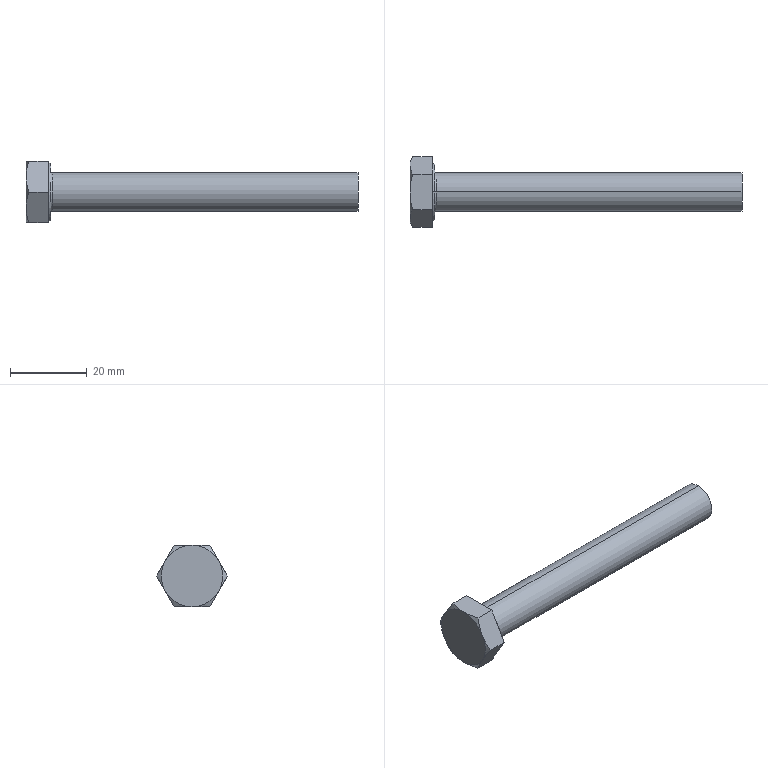Part | SolidWorks | features RevCut 3, Extrusion 1, Fillet 1, LPattern 1, Revolution 1 | 1 solid | 22 faces | box 86.4 x 18.475 x 16 mm | volume 7671 mm3 | plane 10 | cone 8 | torus 2 | cylinder 2 | commonest cylinder face diameters 10 x2
STEP:
#1=CARTESIAN_POINT('',(6.8,0.,5.));
#2=VERTEX_POINT('',#1);
#3=CARTESIAN_POINT('',(6.8,0.,-5.));
#4=VERTEX_POINT('',#3);
#5=CARTESIAN_POINT('',(6.8,0.,0.));
#6=DIRECTION('',(1.,0.,0.));
#7=DIRECTION('',(0.,0.,-1.));
#8=AXIS2_PLACEMENT_3D('',#5,#6,#7);
#9=CIRCLE('',#8,5.);
#10=EDGE_CURVE('',#2,#4,#9,.T.);
#11=ORIENTED_EDGE('',*,*,#10,.F.);
#12=CARTESIAN_POINT('',(6.4,0.,5.4));
#13=VERTEX_POINT('',#12);
#14=CARTESIAN_POINT('',(6.8,0.,5.4));
#15=DIRECTION('',(0.,1.,0.));
#16=DIRECTION('',(0.,0.,1.));
#17=AXIS2_PLACEMENT_3D('',#14,#15,#16);
#18=CIRCLE('',#17,0.4);
#19=EDGE_CURVE('',#2,#13,#18,.T.);
#20=ORIENTED_EDGE('',*,*,#19,.T.);
#21=CARTESIAN_POINT('',(6.4,0.,-5.4));
#22=VERTEX_POINT('',#21);
#23=CARTESIAN_POINT('',(6.4,0.,0.));
#24=DIRECTION('',(-1.,0.,0.));
#25=DIRECTION('',(0.,0.,-1.));
#26=AXIS2_PLACEMENT_3D('',#23,#24,#25);
#27=CIRCLE('',#26,5.4);
#28=EDGE_CURVE('',#22,#13,#27,.T.);
#29=ORIENTED_EDGE('',*,*,#28,.F.);
#30=CARTESIAN_POINT('',(6.8,0.,-5.4));
#31=DIRECTION('',(0.,-1.,0.));
#32=DIRECTION('',(0.,0.,-1.));
#33=AXIS2_PLACEMENT_3D('',#30,#31,#32);
#34=CIRCLE('',#33,0.4);
#35=EDGE_CURVE('',#4,#22,#34,.T.);
#36=ORIENTED_EDGE('',*,*,#35,.F.);
#37=EDGE_LOOP('',(#11,#20,#29,#36));
#38=FACE_OUTER_BOUND('',#37,.T.);
#39=CARTESIAN_POINT('',(6.8,0.,0.));
#40=DIRECTION('',(1.,0.,0.));
#41=DIRECTION('',(0.,0.,-1.));
#42=AXIS2_PLACEMENT_3D('',#39,#40,#41);
#43=TOROIDAL_SURFACE('',#42,5.4,0.4);
#44=ADVANCED_FACE('',(#38),#43,.F.);
#45=CARTESIAN_POINT('',(86.4,0.,5.));
#46=VERTEX_POINT('',#45);
#47=CARTESIAN_POINT('',(86.4,0.,-5.));
#48=VERTEX_POINT('',#47);
#49=CARTESIAN_POINT('',(86.4,0.,0.));
#50=DIRECTION('',(-1.,0.,0.));
#51=DIRECTION('',(0.,0.,1.));
#52=AXIS2_PLACEMENT_3D('',#49,#50,#51);
#53=CIRCLE('',#52,5.);
#54=EDGE_CURVE('',#46,#48,#53,.T.);
#55=ORIENTED_EDGE('',*,*,#54,.T.);
#56=CARTESIAN_POINT('',(0.,0.,-5.));
#57=DIRECTION('',(-1.,0.,0.));
#58=VECTOR('',#57,1000.);
#59=LINE('',#56,#58);
#60=EDGE_CURVE('',#48,#4,#59,.T.);
#61=ORIENTED_EDGE('',*,*,#60,.T.);
#62=CARTESIAN_POINT('',(6.8,0.,0.));
#63=DIRECTION('',(1.,0.,0.));
#64=DIRECTION('',(0.,0.,-1.));
#65=AXIS2_PLACEMENT_3D('',#62,#63,#64);
#66=CIRCLE('',#65,5.);
#67=EDGE_CURVE('',#4,#2,#66,.T.);
#68=ORIENTED_EDGE('',*,*,#67,.T.);
#69=CARTESIAN_POINT('',(0.,0.,5.));
#70=DIRECTION('',(-1.,0.,0.));
#71=VECTOR('',#70,1000.);
#72=LINE('',#69,#71);
#73=EDGE_CURVE('',#46,#2,#72,.T.);
#74=ORIENTED_EDGE('',*,*,#73,.F.);
#75=EDGE_LOOP('',(#55,#61,#68,#74));
#76=FACE_OUTER_BOUND('',#75,.T.);
#77=CARTESIAN_POINT('',(0.,0.,0.));
#78=DIRECTION('',(-1.,0.,0.));
#79=DIRECTION('',(0.,0.,1.));
#80=AXIS2_PLACEMENT_3D('',#77,#78,#79);
#81=CYLINDRICAL_SURFACE('',#80,5.);
#82=ADVANCED_FACE('',(#76),#81,.T.);
#83=CARTESIAN_POINT('',(6.4,0.,7.315));
#84=VERTEX_POINT('',#83);
#85=CARTESIAN_POINT('',(6.4,0.,-7.315));
#86=VERTEX_POINT('',#85);
#87=CARTESIAN_POINT('',(6.4,0.,0.));
#88=DIRECTION('',(-1.,0.,0.));
#89=DIRECTION('',(0.,0.,1.));
#90=AXIS2_PLACEMENT_3D('',#87,#88,#89);
#91=CIRCLE('',#90,7.315);
#92=EDGE_CURVE('',#84,#86,#91,.T.);
#93=ORIENTED_EDGE('',*,*,#92,.T.);
#94=CARTESIAN_POINT('',(5.8,0.,-7.661));
#95=VERTEX_POINT('',#94);
#96=CARTESIAN_POINT('',(5.8,0.,-7.661));
#97=DIRECTION('',(-0.866,0.,-0.5));
#98=VECTOR('',#97,1000.);
#99=LINE('',#96,#98);
#100=EDGE_CURVE('',#86,#95,#99,.T.);
#101=ORIENTED_EDGE('',*,*,#100,.T.);
#102=CARTESIAN_POINT('',(5.8,0.,7.661));
#103=VERTEX_POINT('',#102);
#104=CARTESIAN_POINT('',(5.8,0.,0.));
#105=DIRECTION('',(-1.,0.,0.));
#106=DIRECTION('',(0.,0.,1.));
#107=AXIS2_PLACEMENT_3D('',#104,#105,#106);
#108=CIRCLE('',#107,7.661);
#109=EDGE_CURVE('',#103,#95,#108,.T.);
#110=ORIENTED_EDGE('',*,*,#109,.F.);
#111=CARTESIAN_POINT('',(5.8,0.,7.661));
#112=DIRECTION('',(-0.866,0.,0.5));
#113=VECTOR('',#112,1000.);
#114=LINE('',#111,#113);
#115=EDGE_CURVE('',#84,#103,#114,.T.);
#116=ORIENTED_EDGE('',*,*,#115,.F.);
#117=EDGE_LOOP('',(#93,#101,#110,#116));
#118=FACE_OUTER_BOUND('',#117,.T.);
#119=CARTESIAN_POINT('',(5.8,0.,0.));
#120=DIRECTION('',(-1.,0.,0.));
#121=DIRECTION('',(0.,0.,1.));
#122=AXIS2_PLACEMENT_3D('',#119,#120,#121);
#123=CONICAL_SURFACE('',#122,7.661,0.5236);
#124=ADVANCED_FACE('',(#118),#123,.T.);
#125=CARTESIAN_POINT('',(5.8,4.619,-8.));
#126=VERTEX_POINT('',#125);
#127=CARTESIAN_POINT('',(5.8,9.238,0.));
#128=VERTEX_POINT('',#127);
#129=CARTESIAN_POINT('',(5.8,4.619,-8.));
#130=DIRECTION('',(0.,0.5,0.866));
#131=VECTOR('',#130,1000.);
#132=LINE('',#129,#131);
#133=EDGE_CURVE('',#126,#128,#132,.T.);
#134=ORIENTED_EDGE('',*,*,#133,.F.);
#135=CARTESIAN_POINT('',(0.7145,4.619,-8.));
#136=VERTEX_POINT('',#135);
#137=CARTESIAN_POINT('',(6.4,4.619,-8.));
#138=DIRECTION('',(-1.,0.,0.));
#139=VECTOR('',#138,1000.);
#140=LINE('',#137,#139);
#141=EDGE_CURVE('',#126,#136,#140,.T.);
#142=ORIENTED_EDGE('',*,*,#141,.T.);
#143=CARTESIAN_POINT('',(0.,6.928,-4.));
#144=VERTEX_POINT('',#143);
#145=CARTESIAN_POINT('',(0.,6.928,-4.));
#146=CARTESIAN_POINT('',(0.,6.732,-4.339));
#147=CARTESIAN_POINT('',(0.01689,6.535,-4.68));
#148=CARTESIAN_POINT('',(0.08225,6.146,-5.355));
#149=CARTESIAN_POINT('',(0.1307,5.952,-5.69));
#150=CARTESIAN_POINT('',(0.3174,5.376,-6.689));
#151=CARTESIAN_POINT('',(0.497,4.996,-7.347));
#152=CARTESIAN_POINT('',(0.7145,4.619,-8.));
#153=B_SPLINE_CURVE_WITH_KNOTS('',3,(#145,#146,#147,#148,#149,#150,#151,#152),.UNSPECIFIED.,.F.,.F.,(4,2,2,4),(0.004674,0.005838,0.007002,0.00933),.UNSPECIFIED.);
#154=EDGE_CURVE('',#144,#136,#153,.T.);
#155=ORIENTED_EDGE('',*,*,#154,.F.);
#156=CARTESIAN_POINT('',(0.7145,9.238,0.));
#157=VERTEX_POINT('',#156);
#158=CARTESIAN_POINT('',(0.7145,9.238,0.));
#159=CARTESIAN_POINT('',(0.4964,8.86,-0.6543));
#160=CARTESIAN_POINT('',(0.3167,8.479,-1.313));
#161=CARTESIAN_POINT('',(0.0681,7.71,-2.646));
#162=CARTESIAN_POINT('',(0.,7.322,-3.319));
#163=CARTESIAN_POINT('',(0.,6.928,-4.));
#164=B_SPLINE_CURVE_WITH_KNOTS('',3,(#158,#159,#160,#161,#162,#163),.UNSPECIFIED.,.F.,.F.,(4,2,4),(0.000000238,0.002337,0.004674),.UNSPECIFIED.);
#165=EDGE_CURVE('',#157,#144,#164,.T.);
#166=ORIENTED_EDGE('',*,*,#165,.F.);
#167=CARTESIAN_POINT('',(6.4,9.238,0.));
#168=DIRECTION('',(-1.,0.,0.));
#169=VECTOR('',#168,1000.);
#170=LINE('',#167,#169);
#171=EDGE_CURVE('',#128,#157,#170,.T.);
#172=ORIENTED_EDGE('',*,*,#171,.F.);
#173=EDGE_LOOP('',(#134,#142,#155,#166,#172));
#174=FACE_OUTER_BOUND('',#173,.T.);
#175=CARTESIAN_POINT('',(6.4,4.619,-8.));
#176=DIRECTION('',(0.,-0.866,0.5));
#177=DIRECTION('',(0.,-0.5,-0.866));
#178=AXIS2_PLACEMENT_3D('',#175,#176,#177);
#179=PLANE('',#178);
#180=ADVANCED_FACE('',(#174),#179,.F.);
#181=CARTESIAN_POINT('',(5.8,4.619,8.));
#182=VERTEX_POINT('',#181);
#183=CARTESIAN_POINT('',(5.8,9.238,0.));
#184=DIRECTION('',(0.,-0.5,0.866));
#185=VECTOR('',#184,1000.);
#186=LINE('',#183,#185);
#187=EDGE_CURVE('',#128,#182,#186,.T.);
#188=ORIENTED_EDGE('',*,*,#187,.F.);
#189=ORIENTED_EDGE('',*,*,#171,.T.);
#190=CARTESIAN_POINT('',(0.,6.928,4.));
#191=VERTEX_POINT('',#190);
#192=CARTESIAN_POINT('',(0.,6.928,4.));
#193=CARTESIAN_POINT('',(0.,7.124,3.661));
#194=CARTESIAN_POINT('',(0.01689,7.321,3.32));
#195=CARTESIAN_POINT('',(0.08225,7.711,2.645));
#196=CARTESIAN_POINT('',(0.1307,7.904,2.31));
#197=CARTESIAN_POINT('',(0.3174,8.481,1.311));
#198=CARTESIAN_POINT('',(0.497,8.861,0.6527));
#199=CARTESIAN_POINT('',(0.7145,9.238,0.));
#200=B_SPLINE_CURVE_WITH_KNOTS('',3,(#192,#193,#194,#195,#196,#197,#198,#199),.UNSPECIFIED.,.F.,.F.,(4,2,2,4),(0.004674,0.005838,0.007002,0.00933),.UNSPECIFIED.);
#201=EDGE_CURVE('',#191,#157,#200,.T.);
#202=ORIENTED_EDGE('',*,*,#201,.F.);
#203=CARTESIAN_POINT('',(0.7145,4.619,8.));
#204=VERTEX_POINT('',#203);
#205=CARTESIAN_POINT('',(0.7145,4.619,8.));
#206=CARTESIAN_POINT('',(0.4964,4.997,7.346));
#207=CARTESIAN_POINT('',(0.3167,5.377,6.687));
#208=CARTESIAN_POINT('',(0.0681,6.146,5.354));
#209=CARTESIAN_POINT('',(0.,6.535,4.681));
#210=CARTESIAN_POINT('',(0.,6.928,4.));
#211=B_SPLINE_CURVE_WITH_KNOTS('',3,(#205,#206,#207,#208,#209,#210),.UNSPECIFIED.,.F.,.F.,(4,2,4),(0.000000238,0.002337,0.004674),.UNSPECIFIED.);
#212=EDGE_CURVE('',#204,#191,#211,.T.);
#213=ORIENTED_EDGE('',*,*,#212,.F.);
#214=CARTESIAN_POINT('',(6.4,4.619,8.));
#215=DIRECTION('',(-1.,0.,0.));
#216=VECTOR('',#215,1000.);
#217=LINE('',#214,#216);
#218=EDGE_CURVE('',#182,#204,#217,.T.);
#219=ORIENTED_EDGE('',*,*,#218,.F.);
#220=EDGE_LOOP('',(#188,#189,#202,#213,#219));
#221=FACE_OUTER_BOUND('',#220,.T.);
#222=CARTESIAN_POINT('',(6.4,9.238,0.));
#223=DIRECTION('',(0.,-0.866,-0.5));
#224=DIRECTION('',(0.,0.5,-0.866));
#225=AXIS2_PLACEMENT_3D('',#222,#223,#224);
#226=PLANE('',#225);
#227=ADVANCED_FACE('',(#221),#226,.F.);
#228=CARTESIAN_POINT('',(5.8,-4.619,8.));
#229=VERTEX_POINT('',#228);
#230=CARTESIAN_POINT('',(5.8,4.619,8.));
#231=DIRECTION('',(0.,-1.,0.));
#232=VECTOR('',#231,1000.);
#233=LINE('',#230,#232);
#234=EDGE_CURVE('',#182,#229,#233,.T.);
#235=ORIENTED_EDGE('',*,*,#234,.F.);
#236=ORIENTED_EDGE('',*,*,#218,.T.);
#237=CARTESIAN_POINT('',(0.,0.,8.));
#238=VERTEX_POINT('',#237);
#239=CARTESIAN_POINT('',(0.,0.,8.));
#240=CARTESIAN_POINT('',(0.,0.3913,8.));
#241=CARTESIAN_POINT('',(0.01678,0.7854,8.));
#242=CARTESIAN_POINT('',(0.08286,1.571,8.));
#243=CARTESIAN_POINT('',(0.1318,1.96,8.));
#244=CARTESIAN_POINT('',(0.3194,3.115,8.));
#245=CARTESIAN_POINT('',(0.4988,3.872,8.));
#246=CARTESIAN_POINT('',(0.7145,4.619,8.));
#247=B_SPLINE_CURVE_WITH_KNOTS('',3,(#239,#240,#241,#242,#243,#244,#245,#246),.UNSPECIFIED.,.F.,.F.,(4,2,2,4),(0.01337,0.01454,0.01571,0.01805),.UNSPECIFIED.);
#248=EDGE_CURVE('',#238,#204,#247,.T.);
#249=ORIENTED_EDGE('',*,*,#248,.F.);
#250=CARTESIAN_POINT('',(0.7145,-4.619,8.));
#251=VERTEX_POINT('',#250);
#252=CARTESIAN_POINT('',(0.7145,-4.619,8.));
#253=CARTESIAN_POINT('',(0.4973,-3.866,8.));
#254=CARTESIAN_POINT('',(0.3158,-3.098,8.));
#255=CARTESIAN_POINT('',(0.0673,-1.557,8.));
#256=CARTESIAN_POINT('',(0.,-0.7819,8.));
#257=CARTESIAN_POINT('',(0.,0.,8.));
#258=B_SPLINE_CURVE_WITH_KNOTS('',3,(#252,#253,#254,#255,#256,#257),.UNSPECIFIED.,.F.,.F.,(4,2,4),(0.00869,0.01103,0.01337),.UNSPECIFIED.);
#259=EDGE_CURVE('',#251,#238,#258,.T.);
#260=ORIENTED_EDGE('',*,*,#259,.F.);
#261=CARTESIAN_POINT('',(6.4,-4.619,8.));
#262=DIRECTION('',(-1.,0.,0.));
#263=VECTOR('',#262,1000.);
#264=LINE('',#261,#263);
#265=EDGE_CURVE('',#229,#251,#264,.T.);
#266=ORIENTED_EDGE('',*,*,#265,.F.);
#267=EDGE_LOOP('',(#235,#236,#249,#260,#266));
#268=FACE_OUTER_BOUND('',#267,.T.);
#269=CARTESIAN_POINT('',(6.4,4.619,8.));
#270=DIRECTION('',(0.,0.,-1.));
#271=DIRECTION('',(0.,1.,0.));
#272=AXIS2_PLACEMENT_3D('',#269,#270,#271);
#273=PLANE('',#272);
#274=ADVANCED_FACE('',(#268),#273,.F.);
#275=CARTESIAN_POINT('',(5.8,-9.238,0.));
#276=VERTEX_POINT('',#275);
#277=CARTESIAN_POINT('',(5.8,-9.238,0.));
#278=DIRECTION('',(0.,-0.5,-0.866));
#279=VECTOR('',#278,1000.);
#280=LINE('',#277,#279);
#281=EDGE_CURVE('',#229,#276,#280,.T.);
#282=ORIENTED_EDGE('',*,*,#281,.F.);
#283=ORIENTED_EDGE('',*,*,#265,.T.);
#284=CARTESIAN_POINT('',(0.,-6.928,4.));
#285=VERTEX_POINT('',#284);
#286=CARTESIAN_POINT('',(0.,-6.928,4.));
#287=CARTESIAN_POINT('',(0.,-6.732,4.339));
#288=CARTESIAN_POINT('',(0.01689,-6.535,4.68));
#289=CARTESIAN_POINT('',(0.08225,-6.146,5.355));
#290=CARTESIAN_POINT('',(0.1307,-5.952,5.69));
#291=CARTESIAN_POINT('',(0.3174,-5.376,6.689));
#292=CARTESIAN_POINT('',(0.497,-4.996,7.347));
#293=CARTESIAN_POINT('',(0.7145,-4.619,8.));
#294=B_SPLINE_CURVE_WITH_KNOTS('',3,(#286,#287,#288,#289,#290,#291,#292,#293),.UNSPECIFIED.,.F.,.F.,(4,2,2,4),(0.004674,0.005838,0.007002,0.00933),.UNSPECIFIED.);
#295=EDGE_CURVE('',#285,#251,#294,.T.);
#296=ORIENTED_EDGE('',*,*,#295,.F.);
#297=CARTESIAN_POINT('',(0.7145,-9.238,0.));
#298=VERTEX_POINT('',#297);
#299=CARTESIAN_POINT('',(0.7145,-9.238,0.));
#300=CARTESIAN_POINT('',(0.4964,-8.86,0.6543));
#301=CARTESIAN_POINT('',(0.3167,-8.479,1.313));
#302=CARTESIAN_POINT('',(0.0681,-7.71,2.646));
#303=CARTESIAN_POINT('',(0.,-7.322,3.319));
#304=CARTESIAN_POINT('',(0.,-6.928,4.));
#305=B_SPLINE_CURVE_WITH_KNOTS('',3,(#299,#300,#301,#302,#303,#304),.UNSPECIFIED.,.F.,.F.,(4,2,4),(0.000000238,0.002337,0.004674),.UNSPECIFIED.);
#306=EDGE_CURVE('',#298,#285,#305,.T.);
#307=ORIENTED_EDGE('',*,*,#306,.F.);
#308=CARTESIAN_POINT('',(6.4,-9.238,0.));
#309=DIRECTION('',(-1.,0.,0.));
#310=VECTOR('',#309,1000.);
#311=LINE('',#308,#310);
#312=EDGE_CURVE('',#276,#298,#311,.T.);
#313=ORIENTED_EDGE('',*,*,#312,.F.);
#314=EDGE_LOOP('',(#282,#283,#296,#307,#313));
#315=FACE_OUTER_BOUND('',#314,.T.);
#316=CARTESIAN_POINT('',(6.4,-9.238,0.));
#317=DIRECTION('',(0.,0.866,-0.5));
#318=DIRECTION('',(0.,0.5,0.866));
#319=AXIS2_PLACEMENT_3D('',#316,#317,#318);
#320=PLANE('',#319);
#321=ADVANCED_FACE('',(#315),#320,.F.);
#322=CARTESIAN_POINT('',(5.8,-4.619,-8.));
#323=VERTEX_POINT('',#322);
#324=CARTESIAN_POINT('',(5.8,-4.619,-8.));
#325=DIRECTION('',(0.,0.5,-0.866));
#326=VECTOR('',#325,1000.);
#327=LINE('',#324,#326);
#328=EDGE_CURVE('',#276,#323,#327,.T.);
#329=ORIENTED_EDGE('',*,*,#328,.F.);
#330=ORIENTED_EDGE('',*,*,#312,.T.);
#331=CARTESIAN_POINT('',(0.,-6.928,-4.));
#332=VERTEX_POINT('',#331);
#333=CARTESIAN_POINT('',(0.,-6.928,-4.));
#334=CARTESIAN_POINT('',(0.,-7.124,-3.661));
#335=CARTESIAN_POINT('',(0.01689,-7.321,-3.32));
#336=CARTESIAN_POINT('',(0.08225,-7.711,-2.645));
#337=CARTESIAN_POINT('',(0.1307,-7.904,-2.31));
#338=CARTESIAN_POINT('',(0.3174,-8.481,-1.311));
#339=CARTESIAN_POINT('',(0.497,-8.861,-0.6527));
#340=CARTESIAN_POINT('',(0.7145,-9.238,0.));
#341=B_SPLINE_CURVE_WITH_KNOTS('',3,(#333,#334,#335,#336,#337,#338,#339,#340),.UNSPECIFIED.,.F.,.F.,(4,2,2,4),(0.004674,0.005838,0.007002,0.00933),.UNSPECIFIED.);
#342=EDGE_CURVE('',#332,#298,#341,.T.);
#343=ORIENTED_EDGE('',*,*,#342,.F.);
#344=CARTESIAN_POINT('',(0.7145,-4.619,-8.));
#345=VERTEX_POINT('',#344);
#346=CARTESIAN_POINT('',(0.7145,-4.619,-8.));
#347=CARTESIAN_POINT('',(0.4964,-4.997,-7.346));
#348=CARTESIAN_POINT('',(0.3167,-5.377,-6.687));
#349=CARTESIAN_POINT('',(0.0681,-6.146,-5.354));
#350=CARTESIAN_POINT('',(0.,-6.535,-4.681));
#351=CARTESIAN_POINT('',(0.,-6.928,-4.));
#352=B_SPLINE_CURVE_WITH_KNOTS('',3,(#346,#347,#348,#349,#350,#351),.UNSPECIFIED.,.F.,.F.,(4,2,4),(0.000000238,0.002337,0.004674),.UNSPECIFIED.);
#353=EDGE_CURVE('',#345,#332,#352,.T.);
#354=ORIENTED_EDGE('',*,*,#353,.F.);
#355=CARTESIAN_POINT('',(6.4,-4.619,-8.));
#356=DIRECTION('',(-1.,0.,0.));
#357=VECTOR('',#356,1000.);
#358=LINE('',#355,#357);
#359=EDGE_CURVE('',#323,#345,#358,.T.);
#360=ORIENTED_EDGE('',*,*,#359,.F.);
#361=EDGE_LOOP('',(#329,#330,#343,#354,#360));
#362=FACE_OUTER_BOUND('',#361,.T.);
#363=CARTESIAN_POINT('',(6.4,-4.619,-8.));
#364=DIRECTION('',(0.,0.866,0.5));
#365=DIRECTION('',(0.,-0.5,0.866));
#366=AXIS2_PLACEMENT_3D('',#363,#364,#365);
#367=PLANE('',#366);
#368=ADVANCED_FACE('',(#362),#367,.F.);
#369=CARTESIAN_POINT('',(5.8,4.619,-8.));
#370=DIRECTION('',(0.,1.,0.));
#371=VECTOR('',#370,1000.);
#372=LINE('',#369,#371);
#373=EDGE_CURVE('',#323,#126,#372,.T.);
#374=ORIENTED_EDGE('',*,*,#373,.F.);
#375=ORIENTED_EDGE('',*,*,#359,.T.);
#376=CARTESIAN_POINT('',(0.,0.,-8.));
#377=VERTEX_POINT('',#376);
#378=CARTESIAN_POINT('',(0.,0.,-8.));
#379=CARTESIAN_POINT('',(0.,-0.7819,-8.));
#380=CARTESIAN_POINT('',(0.0673,-1.557,-8.));
#381=CARTESIAN_POINT('',(0.3158,-3.098,-8.));
#382=CARTESIAN_POINT('',(0.4973,-3.866,-8.));
#383=CARTESIAN_POINT('',(0.7145,-4.619,-8.));
#384=B_SPLINE_CURVE_WITH_KNOTS('',3,(#378,#379,#380,#381,#382,#383),.UNSPECIFIED.,.F.,.F.,(4,2,4),(0.02753,0.02987,0.03221),.UNSPECIFIED.);
#385=EDGE_CURVE('',#377,#345,#384,.T.);
#386=ORIENTED_EDGE('',*,*,#385,.F.);
#387=CARTESIAN_POINT('',(0.7145,4.619,-8.));
#388=CARTESIAN_POINT('',(0.4988,3.872,-8.));
#389=CARTESIAN_POINT('',(0.3194,3.115,-8.));
#390=CARTESIAN_POINT('',(0.1318,1.96,-8.));
#391=CARTESIAN_POINT('',(0.08286,1.571,-8.));
#392=CARTESIAN_POINT('',(0.01678,0.7854,-8.));
#393=CARTESIAN_POINT('',(0.,0.3913,-8.));
#394=CARTESIAN_POINT('',(0.,0.,-8.));
#395=B_SPLINE_CURVE_WITH_KNOTS('',3,(#387,#388,#389,#390,#391,#392,#393,#394),.UNSPECIFIED.,.F.,.F.,(4,2,2,4),(0.02285,0.02519,0.02636,0.02753),.UNSPECIFIED.);
#396=EDGE_CURVE('',#136,#377,#395,.T.);
#397=ORIENTED_EDGE('',*,*,#396,.F.);
#398=ORIENTED_EDGE('',*,*,#141,.F.);
#399=EDGE_LOOP('',(#374,#375,#386,#397,#398));
#400=FACE_OUTER_BOUND('',#399,.T.);
#401=CARTESIAN_POINT('',(6.4,4.619,-8.));
#402=DIRECTION('',(0.,0.,1.));
#403=DIRECTION('',(1.,0.,0.));
#404=AXIS2_PLACEMENT_3D('',#401,#402,#403);
#405=PLANE('',#404);
#406=ADVANCED_FACE('',(#400),#405,.F.);
#407=ORIENTED_EDGE('',*,*,#353,.T.);
#408=CARTESIAN_POINT('',(0.,0.,0.));
#409=DIRECTION('',(1.,0.,0.));
#410=DIRECTION('',(0.,0.,-1.));
#411=AXIS2_PLACEMENT_3D('',#408,#409,#410);
#412=CIRCLE('',#411,8.);
#413=EDGE_CURVE('',#332,#377,#412,.T.);
#414=ORIENTED_EDGE('',*,*,#413,.T.);
#415=ORIENTED_EDGE('',*,*,#385,.T.);
#416=EDGE_LOOP('',(#407,#414,#415));
#417=FACE_OUTER_BOUND('',#416,.T.);
#418=CARTESIAN_POINT('',(0.,0.,0.));
#419=DIRECTION('',(1.,0.,0.));
#420=DIRECTION('',(0.,0.,-1.));
#421=AXIS2_PLACEMENT_3D('',#418,#419,#420);
#422=CONICAL_SURFACE('',#421,8.,1.047);
#423=ADVANCED_FACE('',(#417),#422,.T.);
#424=ORIENTED_EDGE('',*,*,#306,.T.);
#425=CARTESIAN_POINT('',(0.,0.,0.));
#426=DIRECTION('',(1.,0.,0.));
#427=DIRECTION('',(0.,0.,-1.));
#428=AXIS2_PLACEMENT_3D('',#425,#426,#427);
#429=CIRCLE('',#428,8.);
#430=EDGE_CURVE('',#285,#332,#429,.T.);
#431=ORIENTED_EDGE('',*,*,#430,.T.);
#432=ORIENTED_EDGE('',*,*,#342,.T.);
#433=EDGE_LOOP('',(#424,#431,#432));
#434=FACE_OUTER_BOUND('',#433,.T.);
#435=CARTESIAN_POINT('',(0.,0.,0.));
#436=DIRECTION('',(1.,0.,0.));
#437=DIRECTION('',(0.,0.,-1.));
#438=AXIS2_PLACEMENT_3D('',#435,#436,#437);
#439=CONICAL_SURFACE('',#438,8.,1.047);
#440=ADVANCED_FACE('',(#434),#439,.T.);
#441=ORIENTED_EDGE('',*,*,#259,.T.);
#442=CARTESIAN_POINT('',(0.,0.,0.));
#443=DIRECTION('',(1.,0.,0.));
#444=DIRECTION('',(0.,0.,-1.));
#445=AXIS2_PLACEMENT_3D('',#442,#443,#444);
#446=CIRCLE('',#445,8.);
#447=EDGE_CURVE('',#238,#285,#446,.T.);
#448=ORIENTED_EDGE('',*,*,#447,.T.);
#449=ORIENTED_EDGE('',*,*,#295,.T.);
#450=EDGE_LOOP('',(#441,#448,#449));
#451=FACE_OUTER_BOUND('',#450,.T.);
#452=CARTESIAN_POINT('',(0.,0.,0.));
#453=DIRECTION('',(1.,0.,0.));
#454=DIRECTION('',(0.,0.,-1.));
#455=AXIS2_PLACEMENT_3D('',#452,#453,#454);
#456=CONICAL_SURFACE('',#455,8.,1.047);
#457=ADVANCED_FACE('',(#451),#456,.T.);
#458=ORIENTED_EDGE('',*,*,#248,.T.);
#459=ORIENTED_EDGE('',*,*,#212,.T.);
#460=CARTESIAN_POINT('',(0.,0.,0.));
#461=DIRECTION('',(-1.,0.,0.));
#462=DIRECTION('',(0.,0.,1.));
#463=AXIS2_PLACEMENT_3D('',#460,#461,#462);
#464=CIRCLE('',#463,8.);
#465=EDGE_CURVE('',#238,#191,#464,.T.);
#466=ORIENTED_EDGE('',*,*,#465,.F.);
#467=EDGE_LOOP('',(#458,#459,#466));
#468=FACE_OUTER_BOUND('',#467,.T.);
#469=CARTESIAN_POINT('',(0.,0.,0.));
#470=DIRECTION('',(1.,0.,0.));
#471=DIRECTION('',(0.,0.,-1.));
#472=AXIS2_PLACEMENT_3D('',#469,#470,#471);
#473=CONICAL_SURFACE('',#472,8.,1.047);
#474=ADVANCED_FACE('',(#468),#473,.T.);
#475=ORIENTED_EDGE('',*,*,#201,.T.);
#476=ORIENTED_EDGE('',*,*,#165,.T.);
#477=CARTESIAN_POINT('',(0.,0.,0.));
#478=DIRECTION('',(1.,0.,0.));
#479=DIRECTION('',(0.,0.,-1.));
#480=AXIS2_PLACEMENT_3D('',#477,#478,#479);
#481=CIRCLE('',#480,8.);
#482=EDGE_CURVE('',#144,#191,#481,.T.);
#483=ORIENTED_EDGE('',*,*,#482,.T.);
#484=EDGE_LOOP('',(#475,#476,#483));
#485=FACE_OUTER_BOUND('',#484,.T.);
#486=CARTESIAN_POINT('',(0.,0.,0.));
#487=DIRECTION('',(1.,0.,0.));
#488=DIRECTION('',(0.,0.,-1.));
#489=AXIS2_PLACEMENT_3D('',#486,#487,#488);
#490=CONICAL_SURFACE('',#489,8.,1.047);
#491=ADVANCED_FACE('',(#485),#490,.T.);
#492=ORIENTED_EDGE('',*,*,#154,.T.);
#493=ORIENTED_EDGE('',*,*,#396,.T.);
#494=CARTESIAN_POINT('',(0.,0.,0.));
#495=DIRECTION('',(1.,0.,0.));
#496=DIRECTION('',(0.,0.,-1.));
#497=AXIS2_PLACEMENT_3D('',#494,#495,#496);
#498=CIRCLE('',#497,8.);
#499=EDGE_CURVE('',#377,#144,#498,.T.);
#500=ORIENTED_EDGE('',*,*,#499,.T.);
#501=EDGE_LOOP('',(#492,#493,#500));
#502=FACE_OUTER_BOUND('',#501,.T.);
#503=CARTESIAN_POINT('',(0.,0.,0.));
#504=DIRECTION('',(1.,0.,0.));
#505=DIRECTION('',(0.,0.,-1.));
#506=AXIS2_PLACEMENT_3D('',#503,#504,#505);
#507=CONICAL_SURFACE('',#506,8.,1.047);
#508=ADVANCED_FACE('',(#502),#507,.T.);
#509=ORIENTED_EDGE('',*,*,#499,.F.);
#510=ORIENTED_EDGE('',*,*,#413,.F.);
#511=ORIENTED_EDGE('',*,*,#430,.F.);
#512=ORIENTED_EDGE('',*,*,#447,.F.);
#513=ORIENTED_EDGE('',*,*,#465,.T.);
#514=ORIENTED_EDGE('',*,*,#482,.F.);
#515=EDGE_LOOP('',(#509,#510,#511,#512,#513,#514));
#516=FACE_OUTER_BOUND('',#515,.T.);
#517=CARTESIAN_POINT('',(0.,9.238,0.));
#518=DIRECTION('',(1.,0.,0.));
#519=DIRECTION('',(0.,0.,-1.));
#520=AXIS2_PLACEMENT_3D('',#517,#518,#519);
#521=PLANE('',#520);
#522=ADVANCED_FACE('',(#516),#521,.F.);
#523=ORIENTED_EDGE('',*,*,#109,.T.);
#524=CARTESIAN_POINT('',(5.8,0.,0.));
#525=DIRECTION('',(-1.,0.,0.));
#526=DIRECTION('',(0.,0.,1.));
#527=AXIS2_PLACEMENT_3D('',#524,#525,#526);
#528=CIRCLE('',#527,7.661);
#529=EDGE_CURVE('',#95,#103,#528,.T.);
#530=ORIENTED_EDGE('',*,*,#529,.T.);
#531=EDGE_LOOP('',(#523,#530));
#532=FACE_BOUND('',#531,.T.);
#533=ORIENTED_EDGE('',*,*,#133,.T.);
#534=ORIENTED_EDGE('',*,*,#187,.T.);
#535=ORIENTED_EDGE('',*,*,#234,.T.);
#536=ORIENTED_EDGE('',*,*,#281,.T.);
#537=ORIENTED_EDGE('',*,*,#328,.T.);
#538=ORIENTED_EDGE('',*,*,#373,.T.);
#539=EDGE_LOOP('',(#533,#534,#535,#536,#537,#538));
#540=FACE_OUTER_BOUND('',#539,.T.);
#541=CARTESIAN_POINT('',(5.8,7.661,0.));
#542=DIRECTION('',(1.,0.,0.));
#543=DIRECTION('',(0.,0.,-1.));
#544=AXIS2_PLACEMENT_3D('',#541,#542,#543);
#545=PLANE('',#544);
#546=ADVANCED_FACE('',(#532,#540),#545,.T.);
#547=ORIENTED_EDGE('',*,*,#100,.F.);
#548=CARTESIAN_POINT('',(6.4,0.,0.));
#549=DIRECTION('',(-1.,0.,0.));
#550=DIRECTION('',(0.,0.,1.));
#551=AXIS2_PLACEMENT_3D('',#548,#549,#550);
#552=CIRCLE('',#551,7.315);
#553=EDGE_CURVE('',#86,#84,#552,.T.);
#554=ORIENTED_EDGE('',*,*,#553,.T.);
#555=ORIENTED_EDGE('',*,*,#115,.T.);
#556=ORIENTED_EDGE('',*,*,#529,.F.);
#557=EDGE_LOOP('',(#547,#554,#555,#556));
#558=FACE_OUTER_BOUND('',#557,.T.);
#559=CARTESIAN_POINT('',(5.8,0.,0.));
#560=DIRECTION('',(-1.,0.,0.));
#561=DIRECTION('',(0.,0.,1.));
#562=AXIS2_PLACEMENT_3D('',#559,#560,#561);
#563=CONICAL_SURFACE('',#562,7.661,0.5236);
#564=ADVANCED_FACE('',(#558),#563,.T.);
#565=ORIENTED_EDGE('',*,*,#54,.F.);
#566=CARTESIAN_POINT('',(86.4,0.,0.));
#567=DIRECTION('',(-1.,0.,0.));
#568=DIRECTION('',(0.,0.,1.));
#569=AXIS2_PLACEMENT_3D('',#566,#567,#568);
#570=CIRCLE('',#569,5.);
#571=EDGE_CURVE('',#48,#46,#570,.T.);
#572=ORIENTED_EDGE('',*,*,#571,.F.);
#573=EDGE_LOOP('',(#565,#572));
#574=FACE_OUTER_BOUND('',#573,.T.);
#575=CARTESIAN_POINT('',(86.4,0.,0.));
#576=DIRECTION('',(-1.,0.,0.));
#577=DIRECTION('',(0.,0.,1.));
#578=AXIS2_PLACEMENT_3D('',#575,#576,#577);
#579=PLANE('',#578);
#580=ADVANCED_FACE('',(#574),#579,.F.);
#581=ORIENTED_EDGE('',*,*,#60,.F.);
#582=ORIENTED_EDGE('',*,*,#571,.T.);
#583=ORIENTED_EDGE('',*,*,#73,.T.);
#584=ORIENTED_EDGE('',*,*,#10,.T.);
#585=EDGE_LOOP('',(#581,#582,#583,#584));
#586=FACE_OUTER_BOUND('',#585,.T.);
#587=CARTESIAN_POINT('',(0.,0.,0.));
#588=DIRECTION('',(-1.,0.,0.));
#589=DIRECTION('',(0.,0.,1.));
#590=AXIS2_PLACEMENT_3D('',#587,#588,#589);
#591=CYLINDRICAL_SURFACE('',#590,5.);
#592=ADVANCED_FACE('',(#586),#591,.T.);
#593=ORIENTED_EDGE('',*,*,#28,.T.);
#594=CARTESIAN_POINT('',(6.4,0.,0.));
#595=DIRECTION('',(-1.,0.,0.));
#596=DIRECTION('',(0.,0.,-1.));
#597=AXIS2_PLACEMENT_3D('',#594,#595,#596);
#598=CIRCLE('',#597,5.4);
#599=EDGE_CURVE('',#13,#22,#598,.T.);
#600=ORIENTED_EDGE('',*,*,#599,.T.);
#601=EDGE_LOOP('',(#593,#600));
#602=FACE_BOUND('',#601,.T.);
#603=ORIENTED_EDGE('',*,*,#92,.F.);
#604=ORIENTED_EDGE('',*,*,#553,.F.);
#605=EDGE_LOOP('',(#603,#604));
#606=FACE_OUTER_BOUND('',#605,.T.);
#607=CARTESIAN_POINT('',(6.4,9.238,0.));
#608=DIRECTION('',(1.,0.,0.));
#609=DIRECTION('',(0.,0.,-1.));
#610=AXIS2_PLACEMENT_3D('',#607,#608,#609);
#611=PLANE('',#610);
#612=ADVANCED_FACE('',(#602,#606),#611,.T.);
#613=ORIENTED_EDGE('',*,*,#19,.F.);
#614=ORIENTED_EDGE('',*,*,#67,.F.);
#615=ORIENTED_EDGE('',*,*,#35,.T.);
#616=ORIENTED_EDGE('',*,*,#599,.F.);
#617=EDGE_LOOP('',(#613,#614,#615,#616));
#618=FACE_OUTER_BOUND('',#617,.T.);
#619=CARTESIAN_POINT('',(6.8,0.,0.));
#620=DIRECTION('',(1.,0.,0.));
#621=DIRECTION('',(0.,0.,-1.));
#622=AXIS2_PLACEMENT_3D('',#619,#620,#621);
#623=TOROIDAL_SURFACE('',#622,5.4,0.4);
#624=ADVANCED_FACE('',(#618),#623,.F.);
#625=CLOSED_SHELL('',(#44,#82,#124,#180,#227,#274,#321,#368,#406,#423,#440,#457,#474,#491,#508,#522,#546,#564,#580,#592,#612,#624));
#626=MANIFOLD_SOLID_BREP('',#625);
#627=CARTESIAN_POINT('',(0.,0.,0.));
#628=DIRECTION('',(0.,0.,1.));
#629=DIRECTION('',(1.,0.,0.));
#630=AXIS2_PLACEMENT_3D('',#627,#628,#629);
#631=(LENGTH_UNIT()NAMED_UNIT(*)SI_UNIT(.MILLI.,.METRE.));
#632=UNCERTAINTY_MEASURE_WITH_UNIT(LENGTH_MEASURE(0.00001),#631,'','');
#633=(NAMED_UNIT(*)PLANE_ANGLE_UNIT()SI_UNIT($,.RADIAN.));
#634=(NAMED_UNIT(*)SI_UNIT($,.STERADIAN.)SOLID_ANGLE_UNIT());
#635=(GEOMETRIC_REPRESENTATION_CONTEXT(3)GLOBAL_UNCERTAINTY_ASSIGNED_CONTEXT((#632))GLOBAL_UNIT_ASSIGNED_CONTEXT((#631,#633,#634))REPRESENTATION_CONTEXT('',''));
#636=ADVANCED_BREP_SHAPE_REPRESENTATION('',(#626,#630),#635);